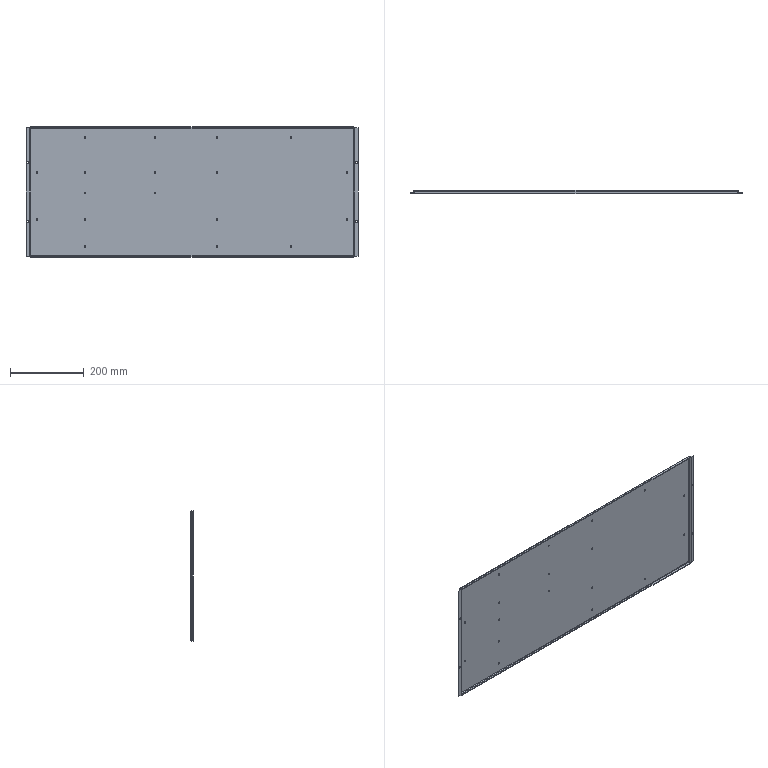Part | STEP file | 1 solid | 94 faces | box 900 x 8 x 353 mm | volume 657092 mm3 | cylinder 56 | plane 38 | commonest cylinder face diameters 4.2 x44 3 x6 7 x6